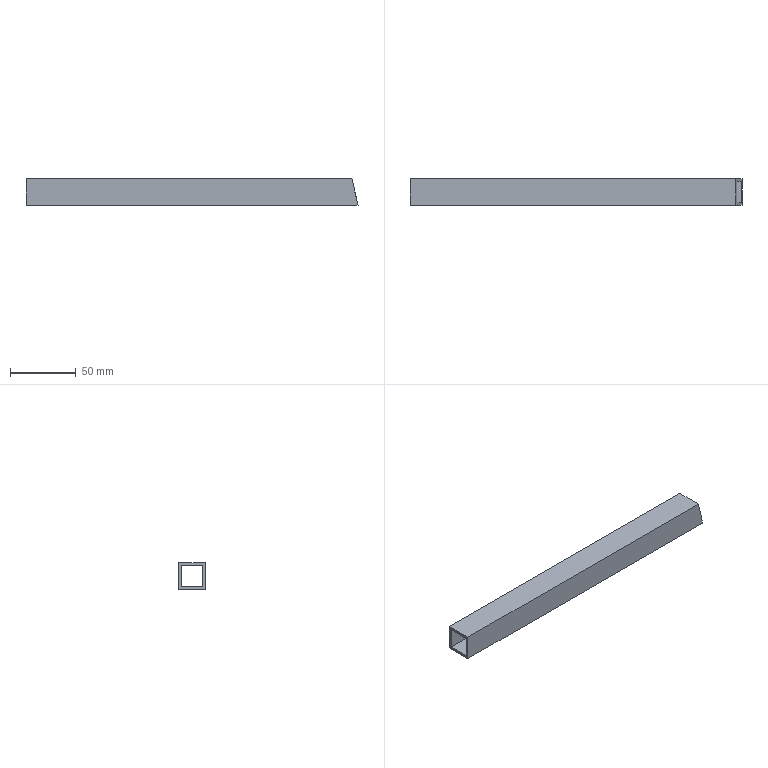Part | NX | features BREP 1 | 1 solid | 10 faces | box 252.949 x 20 x 20 mm | volume 36094 mm3 | plane 10
STEP:
#1=CARTESIAN_POINT('',(1030.163,-696.,401.415));
#2=VERTEX_POINT('',#1);
#3=CARTESIAN_POINT('',(1030.163,-680.,401.415));
#4=VERTEX_POINT('',#3);
#5=CARTESIAN_POINT('',(1030.163,-688.,401.415));
#6=DIRECTION('',(0.,1.,0.));
#7=VECTOR('',#6,1000.);
#8=LINE('',#5,#7);
#9=EDGE_CURVE('',#2,#4,#8,.T.);
#10=ORIENTED_EDGE('',*,*,#9,.F.);
#11=CARTESIAN_POINT('',(1026.492,-696.,417.415));
#12=VERTEX_POINT('',#11);
#13=CARTESIAN_POINT('',(1028.328,-696.,409.415));
#14=DIRECTION('',(-0.2237,0.,0.9747));
#15=VECTOR('',#14,1000.);
#16=LINE('',#13,#15);
#17=EDGE_CURVE('',#2,#12,#16,.T.);
#18=ORIENTED_EDGE('',*,*,#17,.T.);
#19=CARTESIAN_POINT('',(1026.492,-680.,417.415));
#20=VERTEX_POINT('',#19);
#21=CARTESIAN_POINT('',(1026.492,-688.,417.415));
#22=DIRECTION('',(0.,1.,0.));
#23=VECTOR('',#22,1000.);
#24=LINE('',#21,#23);
#25=EDGE_CURVE('',#12,#20,#24,.T.);
#26=ORIENTED_EDGE('',*,*,#25,.T.);
#27=CARTESIAN_POINT('',(1028.328,-680.,409.415));
#28=DIRECTION('',(-0.2237,0.,0.9747));
#29=VECTOR('',#28,1000.);
#30=LINE('',#27,#29);
#31=EDGE_CURVE('',#4,#20,#30,.T.);
#32=ORIENTED_EDGE('',*,*,#31,.F.);
#33=EDGE_LOOP('',(#10,#18,#26,#32));
#34=FACE_BOUND('',#33,.T.);
#35=CARTESIAN_POINT('',(1026.033,-698.,419.415));
#36=VERTEX_POINT('',#35);
#37=CARTESIAN_POINT('',(1026.033,-678.,419.415));
#38=VERTEX_POINT('',#37);
#39=CARTESIAN_POINT('',(1026.033,-688.,419.415));
#40=DIRECTION('',(0.,1.,0.));
#41=VECTOR('',#40,1000.);
#42=LINE('',#39,#41);
#43=EDGE_CURVE('',#36,#38,#42,.T.);
#44=ORIENTED_EDGE('',*,*,#43,.F.);
#45=CARTESIAN_POINT('',(1030.622,-698.,399.415));
#46=VERTEX_POINT('',#45);
#47=CARTESIAN_POINT('',(1026.033,-698.,419.415));
#48=CARTESIAN_POINT('',(1030.622,-698.,399.415));
#49=B_SPLINE_CURVE_WITH_KNOTS('',1,(#47,#48),.UNSPECIFIED.,.F.,.F.,(2,2),(-10.26,10.26),.UNSPECIFIED.);
#50=EDGE_CURVE('',#36,#46,#49,.T.);
#51=ORIENTED_EDGE('',*,*,#50,.T.);
#52=CARTESIAN_POINT('',(1030.622,-678.,399.415));
#53=VERTEX_POINT('',#52);
#54=CARTESIAN_POINT('',(1030.622,-688.,399.415));
#55=DIRECTION('',(0.,1.,0.));
#56=VECTOR('',#55,1000.);
#57=LINE('',#54,#56);
#58=EDGE_CURVE('',#46,#53,#57,.T.);
#59=ORIENTED_EDGE('',*,*,#58,.T.);
#60=CARTESIAN_POINT('',(1030.622,-678.,399.415));
#61=CARTESIAN_POINT('',(1026.033,-678.,419.415));
#62=B_SPLINE_CURVE_WITH_KNOTS('',1,(#60,#61),.UNSPECIFIED.,.F.,.F.,(2,2),(-10.26,10.26),.UNSPECIFIED.);
#63=EDGE_CURVE('',#53,#38,#62,.T.);
#64=ORIENTED_EDGE('',*,*,#63,.T.);
#65=EDGE_LOOP('',(#44,#51,#59,#64));
#66=FACE_BOUND('',#65,.T.);
#67=CARTESIAN_POINT('',(1026.033,-678.,419.415));
#68=DIRECTION('',(0.9747,0.,0.2237));
#69=DIRECTION('',(0.2237,0.,-0.9747));
#70=AXIS2_PLACEMENT_3D('',#67,#68,#69);
#71=PLANE('',#70);
#72=ADVANCED_FACE('',(#34,#66),#71,.T.);
#73=ORIENTED_EDGE('',*,*,#31,.T.);
#74=CARTESIAN_POINT('',(777.673,-680.,417.415));
#75=VERTEX_POINT('',#74);
#76=CARTESIAN_POINT('',(902.083,-680.,417.415));
#77=DIRECTION('',(1.,0.,0.));
#78=VECTOR('',#77,1000.);
#79=LINE('',#76,#78);
#80=EDGE_CURVE('',#75,#20,#79,.T.);
#81=ORIENTED_EDGE('',*,*,#80,.F.);
#82=CARTESIAN_POINT('',(777.673,-680.,401.415));
#83=VERTEX_POINT('',#82);
#84=CARTESIAN_POINT('',(777.673,-680.,401.415));
#85=CARTESIAN_POINT('',(777.673,-680.,404.615));
#86=CARTESIAN_POINT('',(777.673,-680.,407.815));
#87=CARTESIAN_POINT('',(777.673,-680.,411.015));
#88=CARTESIAN_POINT('',(777.673,-680.,414.215));
#89=CARTESIAN_POINT('',(777.673,-680.,417.415));
#90=B_SPLINE_CURVE_WITH_KNOTS('',5,(#84,#85,#86,#87,#88,#89),.UNSPECIFIED.,.F.,.F.,(6,6),(-18.,-2.),.UNSPECIFIED.);
#91=EDGE_CURVE('',#83,#75,#90,.T.);
#92=ORIENTED_EDGE('',*,*,#91,.F.);
#93=CARTESIAN_POINT('',(903.918,-680.,401.415));
#94=DIRECTION('',(1.,0.,0.));
#95=VECTOR('',#94,1000.);
#96=LINE('',#93,#95);
#97=EDGE_CURVE('',#83,#4,#96,.T.);
#98=ORIENTED_EDGE('',*,*,#97,.T.);
#99=EDGE_LOOP('',(#73,#81,#92,#98));
#100=FACE_BOUND('',#99,.T.);
#101=CARTESIAN_POINT('',(1030.163,-680.,401.415));
#102=DIRECTION('',(0.,1.,0.));
#103=DIRECTION('',(-1.,0.,0.));
#104=AXIS2_PLACEMENT_3D('',#101,#102,#103);
#105=PLANE('',#104);
#106=ADVANCED_FACE('',(#100),#105,.F.);
#107=ORIENTED_EDGE('',*,*,#97,.F.);
#108=CARTESIAN_POINT('',(777.673,-696.,401.415));
#109=VERTEX_POINT('',#108);
#110=CARTESIAN_POINT('',(777.673,-696.,401.415));
#111=CARTESIAN_POINT('',(777.673,-692.8,401.415));
#112=CARTESIAN_POINT('',(777.673,-689.6,401.415));
#113=CARTESIAN_POINT('',(777.673,-686.4,401.415));
#114=CARTESIAN_POINT('',(777.673,-683.2,401.415));
#115=CARTESIAN_POINT('',(777.673,-680.,401.415));
#116=B_SPLINE_CURVE_WITH_KNOTS('',5,(#110,#111,#112,#113,#114,#115),.UNSPECIFIED.,.F.,.F.,(6,6),(2.,18.),.UNSPECIFIED.);
#117=EDGE_CURVE('',#109,#83,#116,.T.);
#118=ORIENTED_EDGE('',*,*,#117,.F.);
#119=CARTESIAN_POINT('',(903.918,-696.,401.415));
#120=DIRECTION('',(1.,0.,0.));
#121=VECTOR('',#120,1000.);
#122=LINE('',#119,#121);
#123=EDGE_CURVE('',#109,#2,#122,.T.);
#124=ORIENTED_EDGE('',*,*,#123,.T.);
#125=ORIENTED_EDGE('',*,*,#9,.T.);
#126=EDGE_LOOP('',(#107,#118,#124,#125));
#127=FACE_BOUND('',#126,.T.);
#128=CARTESIAN_POINT('',(766.024,-698.,401.415));
#129=DIRECTION('',(0.,0.,1.));
#130=DIRECTION('',(1.,0.,0.));
#131=AXIS2_PLACEMENT_3D('',#128,#129,#130);
#132=PLANE('',#131);
#133=ADVANCED_FACE('',(#127),#132,.T.);
#134=ORIENTED_EDGE('',*,*,#17,.F.);
#135=ORIENTED_EDGE('',*,*,#123,.F.);
#136=CARTESIAN_POINT('',(777.673,-696.,417.415));
#137=VERTEX_POINT('',#136);
#138=CARTESIAN_POINT('',(777.673,-696.,401.415));
#139=CARTESIAN_POINT('',(777.673,-696.,404.615));
#140=CARTESIAN_POINT('',(777.673,-696.,407.815));
#141=CARTESIAN_POINT('',(777.673,-696.,411.015));
#142=CARTESIAN_POINT('',(777.673,-696.,414.215));
#143=CARTESIAN_POINT('',(777.673,-696.,417.415));
#144=B_SPLINE_CURVE_WITH_KNOTS('',5,(#138,#139,#140,#141,#142,#143),.UNSPECIFIED.,.F.,.F.,(6,6),(-18.,-2.),.UNSPECIFIED.);
#145=EDGE_CURVE('',#109,#137,#144,.T.);
#146=ORIENTED_EDGE('',*,*,#145,.T.);
#147=CARTESIAN_POINT('',(902.083,-696.,417.415));
#148=DIRECTION('',(1.,0.,0.));
#149=VECTOR('',#148,1000.);
#150=LINE('',#147,#149);
#151=EDGE_CURVE('',#137,#12,#150,.T.);
#152=ORIENTED_EDGE('',*,*,#151,.T.);
#153=EDGE_LOOP('',(#134,#135,#146,#152));
#154=FACE_BOUND('',#153,.T.);
#155=CARTESIAN_POINT('',(777.673,-696.,401.415));
#156=DIRECTION('',(0.,-1.,0.));
#157=DIRECTION('',(1.,0.,0.));
#158=AXIS2_PLACEMENT_3D('',#155,#156,#157);
#159=PLANE('',#158);
#160=ADVANCED_FACE('',(#154),#159,.F.);
#161=ORIENTED_EDGE('',*,*,#25,.F.);
#162=ORIENTED_EDGE('',*,*,#151,.F.);
#163=CARTESIAN_POINT('',(777.673,-696.,417.415));
#164=CARTESIAN_POINT('',(777.673,-692.8,417.415));
#165=CARTESIAN_POINT('',(777.673,-689.6,417.415));
#166=CARTESIAN_POINT('',(777.673,-686.4,417.415));
#167=CARTESIAN_POINT('',(777.673,-683.2,417.415));
#168=CARTESIAN_POINT('',(777.673,-680.,417.415));
#169=B_SPLINE_CURVE_WITH_KNOTS('',5,(#163,#164,#165,#166,#167,#168),.UNSPECIFIED.,.F.,.F.,(6,6),(2.,18.),.UNSPECIFIED.);
#170=EDGE_CURVE('',#137,#75,#169,.T.);
#171=ORIENTED_EDGE('',*,*,#170,.T.);
#172=ORIENTED_EDGE('',*,*,#80,.T.);
#173=EDGE_LOOP('',(#161,#162,#171,#172));
#174=FACE_BOUND('',#173,.T.);
#175=CARTESIAN_POINT('',(766.024,-698.,417.415));
#176=DIRECTION('',(0.,0.,1.));
#177=DIRECTION('',(1.,0.,0.));
#178=AXIS2_PLACEMENT_3D('',#175,#176,#177);
#179=PLANE('',#178);
#180=ADVANCED_FACE('',(#174),#179,.F.);
#181=CARTESIAN_POINT('',(777.673,-678.,399.415));
#182=VERTEX_POINT('',#181);
#183=CARTESIAN_POINT('',(904.148,-678.,399.415));
#184=DIRECTION('',(1.,0.,0.));
#185=VECTOR('',#184,1000.);
#186=LINE('',#183,#185);
#187=EDGE_CURVE('',#182,#53,#186,.T.);
#188=ORIENTED_EDGE('',*,*,#187,.F.);
#189=CARTESIAN_POINT('',(777.673,-678.,419.415));
#190=VERTEX_POINT('',#189);
#191=CARTESIAN_POINT('',(777.673,-678.,399.415));
#192=CARTESIAN_POINT('',(777.673,-678.,403.415));
#193=CARTESIAN_POINT('',(777.673,-678.,407.415));
#194=CARTESIAN_POINT('',(777.673,-678.,411.415));
#195=CARTESIAN_POINT('',(777.673,-678.,415.415));
#196=CARTESIAN_POINT('',(777.673,-678.,419.415));
#197=CARTESIAN_POINT('',(777.673,-678.,419.415));
#198=CARTESIAN_POINT('',(777.673,-678.,419.415));
#199=CARTESIAN_POINT('',(777.673,-678.,419.415));
#200=B_SPLINE_CURVE_WITH_KNOTS('',5,(#191,#192,#193,#194,#195,#196,#197,#198,#199),.UNSPECIFIED.,.F.,.F.,(6,3,6),(-20.,-0.000000001,0.0001433),.UNSPECIFIED.);
#201=EDGE_CURVE('',#182,#190,#200,.T.);
#202=ORIENTED_EDGE('',*,*,#201,.T.);
#203=CARTESIAN_POINT('',(901.853,-678.,419.415));
#204=DIRECTION('',(1.,0.,0.));
#205=VECTOR('',#204,1000.);
#206=LINE('',#203,#205);
#207=EDGE_CURVE('',#190,#38,#206,.T.);
#208=ORIENTED_EDGE('',*,*,#207,.T.);
#209=ORIENTED_EDGE('',*,*,#63,.F.);
#210=EDGE_LOOP('',(#188,#202,#208,#209));
#211=FACE_BOUND('',#210,.T.);
#212=CARTESIAN_POINT('',(962.413,-678.,409.415));
#213=DIRECTION('',(0.,1.,0.));
#214=DIRECTION('',(-1.,0.,0.));
#215=AXIS2_PLACEMENT_3D('',#212,#213,#214);
#216=PLANE('',#215);
#217=ADVANCED_FACE('',(#211),#216,.T.);
#218=ORIENTED_EDGE('',*,*,#207,.F.);
#219=CARTESIAN_POINT('',(777.673,-698.,419.415));
#220=VERTEX_POINT('',#219);
#221=CARTESIAN_POINT('',(777.673,-698.,419.415));
#222=CARTESIAN_POINT('',(777.673,-694.,419.415));
#223=CARTESIAN_POINT('',(777.673,-690.,419.415));
#224=CARTESIAN_POINT('',(777.673,-686.,419.415));
#225=CARTESIAN_POINT('',(777.673,-682.,419.415));
#226=CARTESIAN_POINT('',(777.673,-678.,419.415));
#227=B_SPLINE_CURVE_WITH_KNOTS('',5,(#221,#222,#223,#224,#225,#226),.UNSPECIFIED.,.F.,.F.,(6,6),(0.,20.),.UNSPECIFIED.);
#228=EDGE_CURVE('',#220,#190,#227,.T.);
#229=ORIENTED_EDGE('',*,*,#228,.F.);
#230=CARTESIAN_POINT('',(777.673,-698.,419.415));
#231=CARTESIAN_POINT('',(827.345,-698.,419.415));
#232=CARTESIAN_POINT('',(877.017,-698.,419.415));
#233=CARTESIAN_POINT('',(926.689,-698.,419.415));
#234=CARTESIAN_POINT('',(976.361,-698.,419.415));
#235=CARTESIAN_POINT('',(1026.033,-698.,419.415));
#236=B_SPLINE_CURVE_WITH_KNOTS('',5,(#230,#231,#232,#233,#234,#235),.UNSPECIFIED.,.F.,.F.,(6,6),(11.65,260.009),.UNSPECIFIED.);
#237=EDGE_CURVE('',#220,#36,#236,.T.);
#238=ORIENTED_EDGE('',*,*,#237,.T.);
#239=ORIENTED_EDGE('',*,*,#43,.T.);
#240=EDGE_LOOP('',(#218,#229,#238,#239));
#241=FACE_BOUND('',#240,.T.);
#242=CARTESIAN_POINT('',(766.024,-698.,419.415));
#243=DIRECTION('',(0.,0.,1.));
#244=DIRECTION('',(1.,0.,0.));
#245=AXIS2_PLACEMENT_3D('',#242,#243,#244);
#246=PLANE('',#245);
#247=ADVANCED_FACE('',(#241),#246,.T.);
#248=ORIENTED_EDGE('',*,*,#237,.F.);
#249=CARTESIAN_POINT('',(777.673,-698.,399.415));
#250=VERTEX_POINT('',#249);
#251=CARTESIAN_POINT('',(777.673,-698.,399.415));
#252=CARTESIAN_POINT('',(777.673,-698.,403.415));
#253=CARTESIAN_POINT('',(777.673,-698.,407.415));
#254=CARTESIAN_POINT('',(777.673,-698.,411.415));
#255=CARTESIAN_POINT('',(777.673,-698.,415.415));
#256=CARTESIAN_POINT('',(777.673,-698.,419.415));
#257=CARTESIAN_POINT('',(777.673,-698.,419.415));
#258=CARTESIAN_POINT('',(777.673,-698.,419.415));
#259=CARTESIAN_POINT('',(777.673,-698.,419.415));
#260=B_SPLINE_CURVE_WITH_KNOTS('',5,(#251,#252,#253,#254,#255,#256,#257,#258,#259),.UNSPECIFIED.,.F.,.F.,(6,3,6),(-20.,-0.000000001,0.0001433),.UNSPECIFIED.);
#261=EDGE_CURVE('',#250,#220,#260,.T.);
#262=ORIENTED_EDGE('',*,*,#261,.F.);
#263=CARTESIAN_POINT('',(904.148,-698.,399.415));
#264=DIRECTION('',(1.,0.,0.));
#265=VECTOR('',#264,1000.);
#266=LINE('',#263,#265);
#267=EDGE_CURVE('',#250,#46,#266,.T.);
#268=ORIENTED_EDGE('',*,*,#267,.T.);
#269=ORIENTED_EDGE('',*,*,#50,.F.);
#270=EDGE_LOOP('',(#248,#262,#268,#269));
#271=FACE_BOUND('',#270,.T.);
#272=CARTESIAN_POINT('',(962.413,-698.,409.415));
#273=DIRECTION('',(0.,-1.,0.));
#274=DIRECTION('',(1.,0.,0.));
#275=AXIS2_PLACEMENT_3D('',#272,#273,#274);
#276=PLANE('',#275);
#277=ADVANCED_FACE('',(#271),#276,.T.);
#278=ORIENTED_EDGE('',*,*,#58,.F.);
#279=ORIENTED_EDGE('',*,*,#267,.F.);
#280=CARTESIAN_POINT('',(777.673,-698.,399.415));
#281=CARTESIAN_POINT('',(777.673,-694.,399.415));
#282=CARTESIAN_POINT('',(777.673,-690.,399.415));
#283=CARTESIAN_POINT('',(777.673,-686.,399.415));
#284=CARTESIAN_POINT('',(777.673,-682.,399.415));
#285=CARTESIAN_POINT('',(777.673,-678.,399.415));
#286=B_SPLINE_CURVE_WITH_KNOTS('',5,(#280,#281,#282,#283,#284,#285),.UNSPECIFIED.,.F.,.F.,(6,6),(0.,20.),.UNSPECIFIED.);
#287=EDGE_CURVE('',#250,#182,#286,.T.);
#288=ORIENTED_EDGE('',*,*,#287,.T.);
#289=ORIENTED_EDGE('',*,*,#187,.T.);
#290=EDGE_LOOP('',(#278,#279,#288,#289));
#291=FACE_BOUND('',#290,.T.);
#292=CARTESIAN_POINT('',(766.024,-698.,399.415));
#293=DIRECTION('',(0.,0.,1.));
#294=DIRECTION('',(1.,0.,0.));
#295=AXIS2_PLACEMENT_3D('',#292,#293,#294);
#296=PLANE('',#295);
#297=ADVANCED_FACE('',(#291),#296,.F.);
#298=ORIENTED_EDGE('',*,*,#170,.F.);
#299=ORIENTED_EDGE('',*,*,#145,.F.);
#300=ORIENTED_EDGE('',*,*,#117,.T.);
#301=ORIENTED_EDGE('',*,*,#91,.T.);
#302=EDGE_LOOP('',(#298,#299,#300,#301));
#303=FACE_BOUND('',#302,.T.);
#304=ORIENTED_EDGE('',*,*,#287,.F.);
#305=ORIENTED_EDGE('',*,*,#261,.T.);
#306=ORIENTED_EDGE('',*,*,#228,.T.);
#307=ORIENTED_EDGE('',*,*,#201,.F.);
#308=EDGE_LOOP('',(#304,#305,#306,#307));
#309=FACE_BOUND('',#308,.T.);
#310=CARTESIAN_POINT('',(777.673,-688.,636.446));
#311=DIRECTION('',(-1.,0.,0.));
#312=DIRECTION('',(0.,0.,1.));
#313=AXIS2_PLACEMENT_3D('',#310,#311,#312);
#314=PLANE('',#313);
#315=ADVANCED_FACE('',(#303,#309),#314,.T.);
#316=CLOSED_SHELL('',(#72,#106,#133,#160,#180,#217,#247,#277,#297,#315));
#317=MANIFOLD_SOLID_BREP('',#316);
#318=(LENGTH_UNIT()NAMED_UNIT(*)SI_UNIT(.MILLI.,.METRE.));
#319=UNCERTAINTY_MEASURE_WITH_UNIT(LENGTH_MEASURE(0.00001),#318,'','');
#320=(NAMED_UNIT(*)PLANE_ANGLE_UNIT()SI_UNIT($,.RADIAN.));
#321=(NAMED_UNIT(*)SI_UNIT($,.STERADIAN.)SOLID_ANGLE_UNIT());
#322=(GEOMETRIC_REPRESENTATION_CONTEXT(3)GLOBAL_UNCERTAINTY_ASSIGNED_CONTEXT((#319))GLOBAL_UNIT_ASSIGNED_CONTEXT((#318,#320,#321))REPRESENTATION_CONTEXT('',''));
#323=ADVANCED_BREP_SHAPE_REPRESENTATION('',(#317),#322);